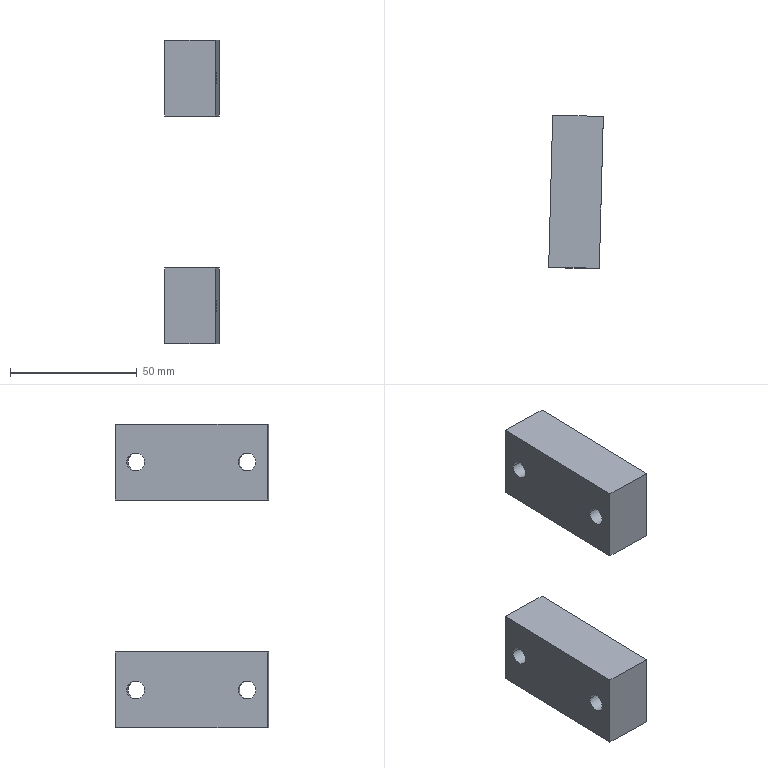Part | STEP file | 666 | 2 solids | 20 faces | box 21.564 x 60.503 x 120 mm | volume 68921 mm3 | plane 12 | cylinder 8 | commonest cylinder face diameters 7 x8